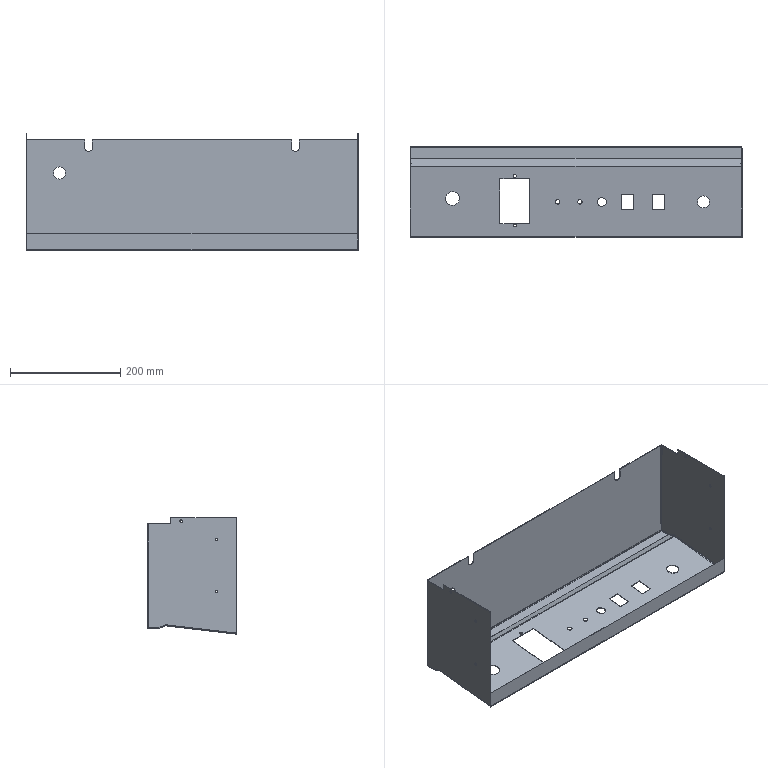Part | SolidWorks | features ICE 6, Cut 3, Fillet 3, ExtruThin 1, MirrorPattern 1 | 1 solid | 91 faces | box 602 x 163.116 x 210.993 mm | volume 271035 mm3 | cylinder 43 | plane 40 | torus 4 | sphere 4 | commonest cylinder face diameters 4.5 x12 4 x11 5.5 x4 8 x4 22 x4 6 x2